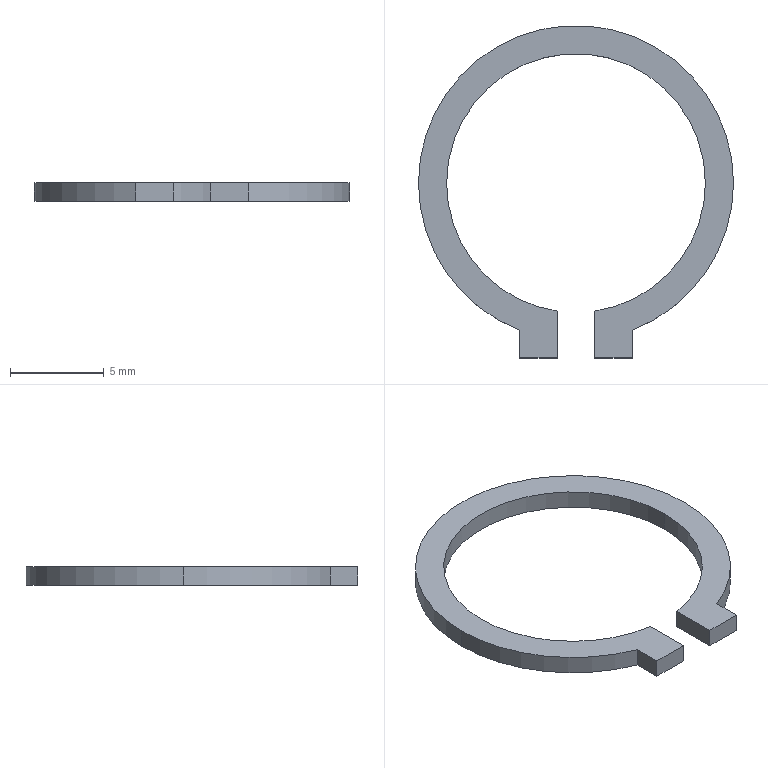Part | STEP file | Outer clip | 1 solid | 14 faces | box 16.8 x 17.727 x 1 mm | volume 73.853 mm3 | plane 8 | cylinder 6 | commonest cylinder face diameters 13.8 x3 16.8 x3
STEP:
#1=CARTESIAN_POINT('',(0.,0.,0.));
#2=DIRECTION('',(0.,0.,1.));
#3=DIRECTION('',(1.,0.,0.));
#4=AXIS2_PLACEMENT_3D('',#1,#2,#3);
#5=CARTESIAN_POINT('',(1.,-6.827,0.));
#6=VERTEX_POINT('',#5);
#7=CARTESIAN_POINT('',(1.,-6.827,1.));
#8=VERTEX_POINT('',#7);
#9=CARTESIAN_POINT('',(1.,-6.827,0.));
#10=DIRECTION('',(0.,0.,1.));
#11=VECTOR('',#10,1.);
#12=LINE('',#9,#11);
#13=CARTESIAN_POINT('',(0.,0.,1.));
#14=DIRECTION('',(0.,0.,-1.));
#15=DIRECTION('',(-1.,0.,0.));
#16=AXIS2_PLACEMENT_3D('',#13,#14,#15);
#17=CYLINDRICAL_SURFACE('',#16,6.9);
#18=CARTESIAN_POINT('',(4.567,1.));
#19=DIRECTION('',(0.,-1.));
#20=VECTOR('',#19,1.);
#21=LINE('',#18,#20);
#22=(GEOMETRIC_REPRESENTATION_CONTEXT(2)PARAMETRIC_REPRESENTATION_CONTEXT()REPRESENTATION_CONTEXT('',''));
#23=DEFINITIONAL_REPRESENTATION('',(#21),#22);
#24=PCURVE('',#17,#23);
#25=CARTESIAN_POINT('',(1.,-5.62,0.));
#26=DIRECTION('',(1.,0.,0.));
#27=DIRECTION('',(0.,1.,0.));
#28=AXIS2_PLACEMENT_3D('',#25,#26,#27);
#29=PLANE('',#28);
#30=CARTESIAN_POINT('',(-1.207,0.));
#31=DIRECTION('',(0.,1.));
#32=VECTOR('',#31,1.);
#33=LINE('',#30,#32);
#34=(GEOMETRIC_REPRESENTATION_CONTEXT(2)PARAMETRIC_REPRESENTATION_CONTEXT()REPRESENTATION_CONTEXT('',''));
#35=DEFINITIONAL_REPRESENTATION('',(#33),#34);
#36=PCURVE('',#29,#35);
#37=SURFACE_CURVE('',#12,(#24,#36),.PCURVE_S1.);
#38=EDGE_CURVE('',#6,#8,#37,.T.);
#39=ORIENTED_EDGE('',*,*,#38,.F.);
#40=CARTESIAN_POINT('',(6.9,0.,0.));
#41=VERTEX_POINT('',#40);
#42=CARTESIAN_POINT('',(0.,0.,0.));
#43=DIRECTION('',(0.,0.,-1.));
#44=DIRECTION('',(-1.,0.,0.));
#45=AXIS2_PLACEMENT_3D('',#42,#43,#44);
#46=CIRCLE('',#45,6.9);
#47=CARTESIAN_POINT('',(0.,1.));
#48=DIRECTION('',(1.,0.));
#49=VECTOR('',#48,1.);
#50=LINE('',#47,#49);
#51=(GEOMETRIC_REPRESENTATION_CONTEXT(2)PARAMETRIC_REPRESENTATION_CONTEXT()REPRESENTATION_CONTEXT('',''));
#52=DEFINITIONAL_REPRESENTATION('',(#50),#51);
#53=PCURVE('',#17,#52);
#54=CARTESIAN_POINT('',(0.,0.,0.));
#55=DIRECTION('',(0.,0.,1.));
#56=DIRECTION('',(1.,0.,0.));
#57=AXIS2_PLACEMENT_3D('',#54,#55,#56);
#58=PLANE('',#57);
#59=CARTESIAN_POINT('',(-6.9,0.));
#60=CARTESIAN_POINT('',(-6.9,11.951));
#61=CARTESIAN_POINT('',(3.45,5.976));
#62=CARTESIAN_POINT('',(13.8,0.));
#63=CARTESIAN_POINT('',(3.45,-5.976));
#64=CARTESIAN_POINT('',(-6.9,-11.951));
#65=CARTESIAN_POINT('',(-6.9,0.));
#66=(BOUNDED_CURVE()B_SPLINE_CURVE(2,(#59,#60,#61,#62,#63,#64,#65),.UNSPECIFIED.,.T.,.F.)B_SPLINE_CURVE_WITH_KNOTS((1,2,2,2,2,1),(-2.094,0.,2.094,4.189,6.283,8.378),.UNSPECIFIED.)CURVE()GEOMETRIC_REPRESENTATION_ITEM()RATIONAL_B_SPLINE_CURVE((1.,0.5,1.,0.5,1.,0.5,1.))REPRESENTATION_ITEM(''));
#67=(GEOMETRIC_REPRESENTATION_CONTEXT(2)PARAMETRIC_REPRESENTATION_CONTEXT()REPRESENTATION_CONTEXT('',''));
#68=DEFINITIONAL_REPRESENTATION('',(#66),#67);
#69=PCURVE('',#58,#68);
#70=SURFACE_CURVE('',#46,(#53,#69),.PCURVE_S1.);
#71=EDGE_CURVE('',#41,#6,#70,.T.);
#72=ORIENTED_EDGE('',*,*,#71,.F.);
#73=CARTESIAN_POINT('',(6.9,0.,1.));
#74=VERTEX_POINT('',#73);
#75=CARTESIAN_POINT('',(6.9,0.,1.));
#76=DIRECTION('',(0.,0.,-1.));
#77=VECTOR('',#76,1.);
#78=LINE('',#75,#77);
#79=CARTESIAN_POINT('',(3.142,0.));
#80=DIRECTION('',(0.,1.));
#81=VECTOR('',#80,1.);
#82=LINE('',#79,#81);
#83=(GEOMETRIC_REPRESENTATION_CONTEXT(2)PARAMETRIC_REPRESENTATION_CONTEXT()REPRESENTATION_CONTEXT('',''));
#84=DEFINITIONAL_REPRESENTATION('',(#82),#83);
#85=PCURVE('',#17,#84);
#86=CARTESIAN_POINT('',(0.,0.,1.));
#87=DIRECTION('',(0.,0.,-1.));
#88=DIRECTION('',(-1.,0.,0.));
#89=AXIS2_PLACEMENT_3D('',#86,#87,#88);
#90=CYLINDRICAL_SURFACE('',#89,6.9);
#91=CARTESIAN_POINT('',(3.142,0.));
#92=DIRECTION('',(0.,1.));
#93=VECTOR('',#92,1.);
#94=LINE('',#91,#93);
#95=(GEOMETRIC_REPRESENTATION_CONTEXT(2)PARAMETRIC_REPRESENTATION_CONTEXT()REPRESENTATION_CONTEXT('',''));
#96=DEFINITIONAL_REPRESENTATION('',(#94),#95);
#97=PCURVE('',#90,#96);
#98=SURFACE_CURVE('',#78,(#85,#97),.PCURVE_S1.);
#99=EDGE_CURVE('',#74,#41,#98,.T.);
#100=ORIENTED_EDGE('',*,*,#99,.F.);
#101=CARTESIAN_POINT('',(0.,0.,1.));
#102=DIRECTION('',(0.,0.,-1.));
#103=DIRECTION('',(-1.,0.,0.));
#104=AXIS2_PLACEMENT_3D('',#101,#102,#103);
#105=CIRCLE('',#104,6.9);
#106=CARTESIAN_POINT('',(0.,0.));
#107=DIRECTION('',(1.,0.));
#108=VECTOR('',#107,1.);
#109=LINE('',#106,#108);
#110=(GEOMETRIC_REPRESENTATION_CONTEXT(2)PARAMETRIC_REPRESENTATION_CONTEXT()REPRESENTATION_CONTEXT('',''));
#111=DEFINITIONAL_REPRESENTATION('',(#109),#110);
#112=PCURVE('',#17,#111);
#113=CARTESIAN_POINT('',(0.,0.,1.));
#114=DIRECTION('',(0.,0.,1.));
#115=DIRECTION('',(1.,0.,0.));
#116=AXIS2_PLACEMENT_3D('',#113,#114,#115);
#117=PLANE('',#116);
#118=CARTESIAN_POINT('',(-6.9,0.));
#119=CARTESIAN_POINT('',(-6.9,11.951));
#120=CARTESIAN_POINT('',(3.45,5.976));
#121=CARTESIAN_POINT('',(13.8,0.));
#122=CARTESIAN_POINT('',(3.45,-5.976));
#123=CARTESIAN_POINT('',(-6.9,-11.951));
#124=CARTESIAN_POINT('',(-6.9,0.));
#125=(BOUNDED_CURVE()B_SPLINE_CURVE(2,(#118,#119,#120,#121,#122,#123,#124),.UNSPECIFIED.,.T.,.F.)B_SPLINE_CURVE_WITH_KNOTS((1,2,2,2,2,1),(-2.094,0.,2.094,4.189,6.283,8.378),.UNSPECIFIED.)CURVE()GEOMETRIC_REPRESENTATION_ITEM()RATIONAL_B_SPLINE_CURVE((1.,0.5,1.,0.5,1.,0.5,1.))REPRESENTATION_ITEM(''));
#126=(GEOMETRIC_REPRESENTATION_CONTEXT(2)PARAMETRIC_REPRESENTATION_CONTEXT()REPRESENTATION_CONTEXT('',''));
#127=DEFINITIONAL_REPRESENTATION('',(#125),#126);
#128=PCURVE('',#117,#127);
#129=SURFACE_CURVE('',#105,(#112,#128),.PCURVE_S1.);
#130=EDGE_CURVE('',#74,#8,#129,.T.);
#131=ORIENTED_EDGE('',*,*,#130,.T.);
#132=EDGE_LOOP('',(#39,#72,#100,#131));
#133=FACE_BOUND('',#132,.F.);
#134=ADVANCED_FACE('',(#133),#17,.F.);
#135=CARTESIAN_POINT('',(-6.9,0.,0.));
#136=VERTEX_POINT('',#135);
#137=CARTESIAN_POINT('',(0.,0.,0.));
#138=DIRECTION('',(0.,0.,-1.));
#139=DIRECTION('',(-1.,0.,0.));
#140=AXIS2_PLACEMENT_3D('',#137,#138,#139);
#141=CIRCLE('',#140,6.9);
#142=CARTESIAN_POINT('',(0.,1.));
#143=DIRECTION('',(1.,0.));
#144=VECTOR('',#143,1.);
#145=LINE('',#142,#144);
#146=(GEOMETRIC_REPRESENTATION_CONTEXT(2)PARAMETRIC_REPRESENTATION_CONTEXT()REPRESENTATION_CONTEXT('',''));
#147=DEFINITIONAL_REPRESENTATION('',(#145),#146);
#148=PCURVE('',#90,#147);
#149=CARTESIAN_POINT('',(-6.9,0.));
#150=CARTESIAN_POINT('',(-6.9,11.951));
#151=CARTESIAN_POINT('',(3.45,5.976));
#152=CARTESIAN_POINT('',(13.8,0.));
#153=CARTESIAN_POINT('',(3.45,-5.976));
#154=CARTESIAN_POINT('',(-6.9,-11.951));
#155=CARTESIAN_POINT('',(-6.9,0.));
#156=(BOUNDED_CURVE()B_SPLINE_CURVE(2,(#149,#150,#151,#152,#153,#154,#155),.UNSPECIFIED.,.T.,.F.)B_SPLINE_CURVE_WITH_KNOTS((1,2,2,2,2,1),(-2.094,0.,2.094,4.189,6.283,8.378),.UNSPECIFIED.)CURVE()GEOMETRIC_REPRESENTATION_ITEM()RATIONAL_B_SPLINE_CURVE((1.,0.5,1.,0.5,1.,0.5,1.))REPRESENTATION_ITEM(''));
#157=(GEOMETRIC_REPRESENTATION_CONTEXT(2)PARAMETRIC_REPRESENTATION_CONTEXT()REPRESENTATION_CONTEXT('',''));
#158=DEFINITIONAL_REPRESENTATION('',(#156),#157);
#159=PCURVE('',#58,#158);
#160=SURFACE_CURVE('',#141,(#148,#159),.PCURVE_S1.);
#161=EDGE_CURVE('',#136,#41,#160,.T.);
#162=ORIENTED_EDGE('',*,*,#161,.F.);
#163=CARTESIAN_POINT('',(-6.9,0.,1.));
#164=VERTEX_POINT('',#163);
#165=CARTESIAN_POINT('',(-6.9,0.,1.));
#166=DIRECTION('',(0.,0.,-1.));
#167=VECTOR('',#166,1.);
#168=LINE('',#165,#167);
#169=CARTESIAN_POINT('',(0.,0.));
#170=DIRECTION('',(0.,1.));
#171=VECTOR('',#170,1.);
#172=LINE('',#169,#171);
#173=(GEOMETRIC_REPRESENTATION_CONTEXT(2)PARAMETRIC_REPRESENTATION_CONTEXT()REPRESENTATION_CONTEXT('',''));
#174=DEFINITIONAL_REPRESENTATION('',(#172),#173);
#175=PCURVE('',#90,#174);
#176=CARTESIAN_POINT('',(0.,0.,1.));
#177=DIRECTION('',(0.,0.,-1.));
#178=DIRECTION('',(-1.,0.,0.));
#179=AXIS2_PLACEMENT_3D('',#176,#177,#178);
#180=CYLINDRICAL_SURFACE('',#179,6.9);
#181=CARTESIAN_POINT('',(6.283,0.));
#182=DIRECTION('',(0.,1.));
#183=VECTOR('',#182,1.);
#184=LINE('',#181,#183);
#185=(GEOMETRIC_REPRESENTATION_CONTEXT(2)PARAMETRIC_REPRESENTATION_CONTEXT()REPRESENTATION_CONTEXT('',''));
#186=DEFINITIONAL_REPRESENTATION('',(#184),#185);
#187=PCURVE('',#180,#186);
#188=SURFACE_CURVE('',#168,(#175,#187),.PCURVE_S1.);
#189=EDGE_CURVE('',#164,#136,#188,.T.);
#190=ORIENTED_EDGE('',*,*,#189,.F.);
#191=CARTESIAN_POINT('',(0.,0.,1.));
#192=DIRECTION('',(0.,0.,-1.));
#193=DIRECTION('',(-1.,0.,0.));
#194=AXIS2_PLACEMENT_3D('',#191,#192,#193);
#195=CIRCLE('',#194,6.9);
#196=CARTESIAN_POINT('',(0.,0.));
#197=DIRECTION('',(1.,0.));
#198=VECTOR('',#197,1.);
#199=LINE('',#196,#198);
#200=(GEOMETRIC_REPRESENTATION_CONTEXT(2)PARAMETRIC_REPRESENTATION_CONTEXT()REPRESENTATION_CONTEXT('',''));
#201=DEFINITIONAL_REPRESENTATION('',(#199),#200);
#202=PCURVE('',#90,#201);
#203=CARTESIAN_POINT('',(-6.9,0.));
#204=CARTESIAN_POINT('',(-6.9,11.951));
#205=CARTESIAN_POINT('',(3.45,5.976));
#206=CARTESIAN_POINT('',(13.8,0.));
#207=CARTESIAN_POINT('',(3.45,-5.976));
#208=CARTESIAN_POINT('',(-6.9,-11.951));
#209=CARTESIAN_POINT('',(-6.9,0.));
#210=(BOUNDED_CURVE()B_SPLINE_CURVE(2,(#203,#204,#205,#206,#207,#208,#209),.UNSPECIFIED.,.T.,.F.)B_SPLINE_CURVE_WITH_KNOTS((1,2,2,2,2,1),(-2.094,0.,2.094,4.189,6.283,8.378),.UNSPECIFIED.)CURVE()GEOMETRIC_REPRESENTATION_ITEM()RATIONAL_B_SPLINE_CURVE((1.,0.5,1.,0.5,1.,0.5,1.))REPRESENTATION_ITEM(''));
#211=(GEOMETRIC_REPRESENTATION_CONTEXT(2)PARAMETRIC_REPRESENTATION_CONTEXT()REPRESENTATION_CONTEXT('',''));
#212=DEFINITIONAL_REPRESENTATION('',(#210),#211);
#213=PCURVE('',#117,#212);
#214=SURFACE_CURVE('',#195,(#202,#213),.PCURVE_S1.);
#215=EDGE_CURVE('',#164,#74,#214,.T.);
#216=ORIENTED_EDGE('',*,*,#215,.T.);
#217=ORIENTED_EDGE('',*,*,#99,.T.);
#218=EDGE_LOOP('',(#162,#190,#216,#217));
#219=FACE_BOUND('',#218,.F.);
#220=ADVANCED_FACE('',(#219),#90,.F.);
#221=CARTESIAN_POINT('',(-8.4,0.,1.));
#222=VERTEX_POINT('',#221);
#223=CARTESIAN_POINT('',(8.4,0.,1.));
#224=VERTEX_POINT('',#223);
#225=CARTESIAN_POINT('',(0.,0.,1.));
#226=DIRECTION('',(0.,0.,-1.));
#227=DIRECTION('',(-1.,0.,0.));
#228=AXIS2_PLACEMENT_3D('',#225,#226,#227);
#229=CIRCLE('',#228,8.4);
#230=CARTESIAN_POINT('',(0.,0.,1.));
#231=DIRECTION('',(0.,0.,-1.));
#232=DIRECTION('',(-1.,0.,0.));
#233=AXIS2_PLACEMENT_3D('',#230,#231,#232);
#234=CYLINDRICAL_SURFACE('',#233,8.4);
#235=CARTESIAN_POINT('',(0.,0.));
#236=DIRECTION('',(1.,0.));
#237=VECTOR('',#236,1.);
#238=LINE('',#235,#237);
#239=(GEOMETRIC_REPRESENTATION_CONTEXT(2)PARAMETRIC_REPRESENTATION_CONTEXT()REPRESENTATION_CONTEXT('',''));
#240=DEFINITIONAL_REPRESENTATION('',(#238),#239);
#241=PCURVE('',#234,#240);
#242=CARTESIAN_POINT('',(-8.4,0.));
#243=CARTESIAN_POINT('',(-8.4,14.549));
#244=CARTESIAN_POINT('',(4.2,7.275));
#245=CARTESIAN_POINT('',(16.8,0.));
#246=CARTESIAN_POINT('',(4.2,-7.275));
#247=CARTESIAN_POINT('',(-8.4,-14.549));
#248=CARTESIAN_POINT('',(-8.4,0.));
#249=(BOUNDED_CURVE()B_SPLINE_CURVE(2,(#242,#243,#244,#245,#246,#247,#248),.UNSPECIFIED.,.T.,.F.)B_SPLINE_CURVE_WITH_KNOTS((1,2,2,2,2,1),(-2.094,0.,2.094,4.189,6.283,8.378),.UNSPECIFIED.)CURVE()GEOMETRIC_REPRESENTATION_ITEM()RATIONAL_B_SPLINE_CURVE((1.,0.5,1.,0.5,1.,0.5,1.))REPRESENTATION_ITEM(''));
#250=(GEOMETRIC_REPRESENTATION_CONTEXT(2)PARAMETRIC_REPRESENTATION_CONTEXT()REPRESENTATION_CONTEXT('',''));
#251=DEFINITIONAL_REPRESENTATION('',(#249),#250);
#252=PCURVE('',#117,#251);
#253=SURFACE_CURVE('',#229,(#241,#252),.PCURVE_S1.);
#254=EDGE_CURVE('',#222,#224,#253,.T.);
#255=ORIENTED_EDGE('',*,*,#254,.T.);
#256=CARTESIAN_POINT('',(8.4,0.,0.));
#257=VERTEX_POINT('',#256);
#258=CARTESIAN_POINT('',(8.4,0.,1.));
#259=DIRECTION('',(0.,0.,-1.));
#260=VECTOR('',#259,1.);
#261=LINE('',#258,#260);
#262=CARTESIAN_POINT('',(3.142,0.));
#263=DIRECTION('',(0.,1.));
#264=VECTOR('',#263,1.);
#265=LINE('',#262,#264);
#266=(GEOMETRIC_REPRESENTATION_CONTEXT(2)PARAMETRIC_REPRESENTATION_CONTEXT()REPRESENTATION_CONTEXT('',''));
#267=DEFINITIONAL_REPRESENTATION('',(#265),#266);
#268=PCURVE('',#234,#267);
#269=CARTESIAN_POINT('',(0.,0.,1.));
#270=DIRECTION('',(0.,0.,-1.));
#271=DIRECTION('',(-1.,0.,0.));
#272=AXIS2_PLACEMENT_3D('',#269,#270,#271);
#273=CYLINDRICAL_SURFACE('',#272,8.4);
#274=CARTESIAN_POINT('',(3.142,0.));
#275=DIRECTION('',(0.,1.));
#276=VECTOR('',#275,1.);
#277=LINE('',#274,#276);
#278=(GEOMETRIC_REPRESENTATION_CONTEXT(2)PARAMETRIC_REPRESENTATION_CONTEXT()REPRESENTATION_CONTEXT('',''));
#279=DEFINITIONAL_REPRESENTATION('',(#277),#278);
#280=PCURVE('',#273,#279);
#281=SURFACE_CURVE('',#261,(#268,#280),.PCURVE_S1.);
#282=EDGE_CURVE('',#224,#257,#281,.T.);
#283=ORIENTED_EDGE('',*,*,#282,.T.);
#284=CARTESIAN_POINT('',(-8.4,0.,0.));
#285=VERTEX_POINT('',#284);
#286=CARTESIAN_POINT('',(0.,0.,0.));
#287=DIRECTION('',(0.,0.,1.));
#288=DIRECTION('',(-1.,0.,0.));
#289=AXIS2_PLACEMENT_3D('',#286,#287,#288);
#290=CIRCLE('',#289,8.4);
#291=CARTESIAN_POINT('',(6.283,1.));
#292=DIRECTION('',(-1.,0.));
#293=VECTOR('',#292,1.);
#294=LINE('',#291,#293);
#295=(GEOMETRIC_REPRESENTATION_CONTEXT(2)PARAMETRIC_REPRESENTATION_CONTEXT()REPRESENTATION_CONTEXT('',''));
#296=DEFINITIONAL_REPRESENTATION('',(#294),#295);
#297=PCURVE('',#234,#296);
#298=CARTESIAN_POINT('',(0.,0.));
#299=DIRECTION('',(-1.,0.));
#300=AXIS2_PLACEMENT_2D('',#298,#299);
#301=CIRCLE('',#300,8.4);
#302=(GEOMETRIC_REPRESENTATION_CONTEXT(2)PARAMETRIC_REPRESENTATION_CONTEXT()REPRESENTATION_CONTEXT('',''));
#303=DEFINITIONAL_REPRESENTATION('',(#301),#302);
#304=PCURVE('',#58,#303);
#305=SURFACE_CURVE('',#290,(#297,#304),.PCURVE_S1.);
#306=EDGE_CURVE('',#257,#285,#305,.T.);
#307=ORIENTED_EDGE('',*,*,#306,.T.);
#308=CARTESIAN_POINT('',(-8.4,0.,1.));
#309=DIRECTION('',(0.,0.,-1.));
#310=VECTOR('',#309,1.);
#311=LINE('',#308,#310);
#312=CARTESIAN_POINT('',(0.,0.));
#313=DIRECTION('',(0.,1.));
#314=VECTOR('',#313,1.);
#315=LINE('',#312,#314);
#316=(GEOMETRIC_REPRESENTATION_CONTEXT(2)PARAMETRIC_REPRESENTATION_CONTEXT()REPRESENTATION_CONTEXT('',''));
#317=DEFINITIONAL_REPRESENTATION('',(#315),#316);
#318=PCURVE('',#234,#317);
#319=CARTESIAN_POINT('',(0.,0.,1.));
#320=DIRECTION('',(0.,0.,-1.));
#321=DIRECTION('',(-1.,0.,0.));
#322=AXIS2_PLACEMENT_3D('',#319,#320,#321);
#323=CYLINDRICAL_SURFACE('',#322,8.4);
#324=CARTESIAN_POINT('',(6.283,0.));
#325=DIRECTION('',(0.,1.));
#326=VECTOR('',#325,1.);
#327=LINE('',#324,#326);
#328=(GEOMETRIC_REPRESENTATION_CONTEXT(2)PARAMETRIC_REPRESENTATION_CONTEXT()REPRESENTATION_CONTEXT('',''));
#329=DEFINITIONAL_REPRESENTATION('',(#327),#328);
#330=PCURVE('',#323,#329);
#331=SURFACE_CURVE('',#311,(#318,#330),.PCURVE_S1.);
#332=EDGE_CURVE('',#222,#285,#331,.T.);
#333=ORIENTED_EDGE('',*,*,#332,.F.);
#334=EDGE_LOOP('',(#255,#283,#307,#333));
#335=FACE_BOUND('',#334,.T.);
#336=ADVANCED_FACE('',(#335),#234,.T.);
#337=CARTESIAN_POINT('',(-3.,-7.846,1.));
#338=VERTEX_POINT('',#337);
#339=CARTESIAN_POINT('',(0.,0.,1.));
#340=DIRECTION('',(0.,0.,-1.));
#341=DIRECTION('',(-1.,0.,0.));
#342=AXIS2_PLACEMENT_3D('',#339,#340,#341);
#343=CIRCLE('',#342,8.4);
#344=CARTESIAN_POINT('',(0.,0.));
#345=DIRECTION('',(1.,0.));
#346=VECTOR('',#345,1.);
#347=LINE('',#344,#346);
#348=(GEOMETRIC_REPRESENTATION_CONTEXT(2)PARAMETRIC_REPRESENTATION_CONTEXT()REPRESENTATION_CONTEXT('',''));
#349=DEFINITIONAL_REPRESENTATION('',(#347),#348);
#350=PCURVE('',#323,#349);
#351=CARTESIAN_POINT('',(-8.4,0.));
#352=CARTESIAN_POINT('',(-8.4,14.549));
#353=CARTESIAN_POINT('',(4.2,7.275));
#354=CARTESIAN_POINT('',(16.8,0.));
#355=CARTESIAN_POINT('',(4.2,-7.275));
#356=CARTESIAN_POINT('',(-8.4,-14.549));
#357=CARTESIAN_POINT('',(-8.4,0.));
#358=(BOUNDED_CURVE()B_SPLINE_CURVE(2,(#351,#352,#353,#354,#355,#356,#357),.UNSPECIFIED.,.T.,.F.)B_SPLINE_CURVE_WITH_KNOTS((1,2,2,2,2,1),(-2.094,0.,2.094,4.189,6.283,8.378),.UNSPECIFIED.)CURVE()GEOMETRIC_REPRESENTATION_ITEM()RATIONAL_B_SPLINE_CURVE((1.,0.5,1.,0.5,1.,0.5,1.))REPRESENTATION_ITEM(''));
#359=(GEOMETRIC_REPRESENTATION_CONTEXT(2)PARAMETRIC_REPRESENTATION_CONTEXT()REPRESENTATION_CONTEXT('',''));
#360=DEFINITIONAL_REPRESENTATION('',(#358),#359);
#361=PCURVE('',#117,#360);
#362=SURFACE_CURVE('',#343,(#350,#361),.PCURVE_S1.);
#363=EDGE_CURVE('',#338,#222,#362,.T.);
#364=ORIENTED_EDGE('',*,*,#363,.T.);
#365=ORIENTED_EDGE('',*,*,#332,.T.);
#366=CARTESIAN_POINT('',(-3.,-7.846,0.));
#367=VERTEX_POINT('',#366);
#368=CARTESIAN_POINT('',(0.,0.,0.));
#369=DIRECTION('',(0.,0.,1.));
#370=DIRECTION('',(-1.,0.,0.));
#371=AXIS2_PLACEMENT_3D('',#368,#369,#370);
#372=CIRCLE('',#371,8.4);
#373=CARTESIAN_POINT('',(6.283,1.));
#374=DIRECTION('',(-1.,0.));
#375=VECTOR('',#374,1.);
#376=LINE('',#373,#375);
#377=(GEOMETRIC_REPRESENTATION_CONTEXT(2)PARAMETRIC_REPRESENTATION_CONTEXT()REPRESENTATION_CONTEXT('',''));
#378=DEFINITIONAL_REPRESENTATION('',(#376),#377);
#379=PCURVE('',#323,#378);
#380=CARTESIAN_POINT('',(0.,0.));
#381=DIRECTION('',(-1.,0.));
#382=AXIS2_PLACEMENT_2D('',#380,#381);
#383=CIRCLE('',#382,8.4);
#384=(GEOMETRIC_REPRESENTATION_CONTEXT(2)PARAMETRIC_REPRESENTATION_CONTEXT()REPRESENTATION_CONTEXT('',''));
#385=DEFINITIONAL_REPRESENTATION('',(#383),#384);
#386=PCURVE('',#58,#385);
#387=SURFACE_CURVE('',#372,(#379,#386),.PCURVE_S1.);
#388=EDGE_CURVE('',#285,#367,#387,.T.);
#389=ORIENTED_EDGE('',*,*,#388,.T.);
#390=CARTESIAN_POINT('',(-3.,-7.846,0.));
#391=DIRECTION('',(0.,0.,-1.));
#392=VECTOR('',#391,1.);
#393=LINE('',#390,#392);
#394=CARTESIAN_POINT('',(5.078,1.));
#395=DIRECTION('',(0.,1.));
#396=VECTOR('',#395,1.);
#397=LINE('',#394,#396);
#398=(GEOMETRIC_REPRESENTATION_CONTEXT(2)PARAMETRIC_REPRESENTATION_CONTEXT()REPRESENTATION_CONTEXT('',''));
#399=DEFINITIONAL_REPRESENTATION('',(#397),#398);
#400=PCURVE('',#323,#399);
#401=CARTESIAN_POINT('',(-3.,-6.827,0.));
#402=DIRECTION('',(-1.,0.,0.));
#403=DIRECTION('',(0.,-1.,0.));
#404=AXIS2_PLACEMENT_3D('',#401,#402,#403);
#405=PLANE('',#404);
#406=CARTESIAN_POINT('',(1.019,0.));
#407=DIRECTION('',(0.,-1.));
#408=VECTOR('',#407,1.);
#409=LINE('',#406,#408);
#410=(GEOMETRIC_REPRESENTATION_CONTEXT(2)PARAMETRIC_REPRESENTATION_CONTEXT()REPRESENTATION_CONTEXT('',''));
#411=DEFINITIONAL_REPRESENTATION('',(#409),#410);
#412=PCURVE('',#405,#411);
#413=SURFACE_CURVE('',#393,(#400,#412),.PCURVE_S1.);
#414=EDGE_CURVE('',#338,#367,#413,.T.);
#415=ORIENTED_EDGE('',*,*,#414,.F.);
#416=EDGE_LOOP('',(#364,#365,#389,#415));
#417=FACE_BOUND('',#416,.T.);
#418=ADVANCED_FACE('',(#417),#323,.T.);
#419=CARTESIAN_POINT('',(1.,-9.327,0.));
#420=VERTEX_POINT('',#419);
#421=CARTESIAN_POINT('',(1.,0.,0.));
#422=DIRECTION('',(0.,-1.,0.));
#423=VECTOR('',#422,1.);
#424=LINE('',#421,#423);
#425=CARTESIAN_POINT('',(1.,0.));
#426=DIRECTION('',(0.,-1.));
#427=VECTOR('',#426,1.);
#428=LINE('',#425,#427);
#429=(GEOMETRIC_REPRESENTATION_CONTEXT(2)PARAMETRIC_REPRESENTATION_CONTEXT()REPRESENTATION_CONTEXT('',''));
#430=DEFINITIONAL_REPRESENTATION('',(#428),#429);
#431=PCURVE('',#58,#430);
#432=CARTESIAN_POINT('',(5.62,0.));
#433=DIRECTION('',(-1.,0.));
#434=VECTOR('',#433,1.);
#435=LINE('',#432,#434);
#436=(GEOMETRIC_REPRESENTATION_CONTEXT(2)PARAMETRIC_REPRESENTATION_CONTEXT()REPRESENTATION_CONTEXT('',''));
#437=DEFINITIONAL_REPRESENTATION('',(#435),#436);
#438=PCURVE('',#29,#437);
#439=SURFACE_CURVE('',#424,(#431,#438),.PCURVE_S1.);
#440=EDGE_CURVE('',#6,#420,#439,.T.);
#441=ORIENTED_EDGE('',*,*,#440,.F.);
#442=ORIENTED_EDGE('',*,*,#71,.F.);
#443=ORIENTED_EDGE('',*,*,#161,.F.);
#444=CARTESIAN_POINT('',(-1.,-6.827,0.));
#445=VERTEX_POINT('',#444);
#446=CARTESIAN_POINT('',(0.,0.,0.));
#447=DIRECTION('',(0.,0.,-1.));
#448=DIRECTION('',(-1.,0.,0.));
#449=AXIS2_PLACEMENT_3D('',#446,#447,#448);
#450=CIRCLE('',#449,6.9);
#451=CARTESIAN_POINT('',(-6.9,0.));
#452=CARTESIAN_POINT('',(-6.9,11.951));
#453=CARTESIAN_POINT('',(3.45,5.976));
#454=CARTESIAN_POINT('',(13.8,0.));
#455=CARTESIAN_POINT('',(3.45,-5.976));
#456=CARTESIAN_POINT('',(-6.9,-11.951));
#457=CARTESIAN_POINT('',(-6.9,0.));
#458=(BOUNDED_CURVE()B_SPLINE_CURVE(2,(#451,#452,#453,#454,#455,#456,#457),.UNSPECIFIED.,.T.,.F.)B_SPLINE_CURVE_WITH_KNOTS((1,2,2,2,2,1),(-2.094,0.,2.094,4.189,6.283,8.378),.UNSPECIFIED.)CURVE()GEOMETRIC_REPRESENTATION_ITEM()RATIONAL_B_SPLINE_CURVE((1.,0.5,1.,0.5,1.,0.5,1.))REPRESENTATION_ITEM(''));
#459=(GEOMETRIC_REPRESENTATION_CONTEXT(2)PARAMETRIC_REPRESENTATION_CONTEXT()REPRESENTATION_CONTEXT('',''));
#460=DEFINITIONAL_REPRESENTATION('',(#458),#459);
#461=PCURVE('',#58,#460);
#462=CARTESIAN_POINT('',(0.,1.));
#463=DIRECTION('',(1.,0.));
#464=VECTOR('',#463,1.);
#465=LINE('',#462,#464);
#466=(GEOMETRIC_REPRESENTATION_CONTEXT(2)PARAMETRIC_REPRESENTATION_CONTEXT()REPRESENTATION_CONTEXT('',''));
#467=DEFINITIONAL_REPRESENTATION('',(#465),#466);
#468=PCURVE('',#180,#467);
#469=SURFACE_CURVE('',#450,(#461,#468),.PCURVE_S1.);
#470=EDGE_CURVE('',#445,#136,#469,.T.);
#471=ORIENTED_EDGE('',*,*,#470,.F.);
#472=CARTESIAN_POINT('',(-1.,-9.327,0.));
#473=VERTEX_POINT('',#472);
#474=CARTESIAN_POINT('',(-1.,0.,0.));
#475=DIRECTION('',(0.,1.,0.));
#476=VECTOR('',#475,1.);
#477=LINE('',#474,#476);
#478=CARTESIAN_POINT('',(-1.,0.));
#479=DIRECTION('',(0.,1.));
#480=VECTOR('',#479,1.);
#481=LINE('',#478,#480);
#482=(GEOMETRIC_REPRESENTATION_CONTEXT(2)PARAMETRIC_REPRESENTATION_CONTEXT()REPRESENTATION_CONTEXT('',''));
#483=DEFINITIONAL_REPRESENTATION('',(#481),#482);
#484=PCURVE('',#58,#483);
#485=CARTESIAN_POINT('',(-1.,-5.62,0.));
#486=DIRECTION('',(-1.,0.,0.));
#487=DIRECTION('',(0.,-1.,0.));
#488=AXIS2_PLACEMENT_3D('',#485,#486,#487);
#489=PLANE('',#488);
#490=CARTESIAN_POINT('',(-5.62,0.));
#491=DIRECTION('',(-1.,0.));
#492=VECTOR('',#491,1.);
#493=LINE('',#490,#492);
#494=(GEOMETRIC_REPRESENTATION_CONTEXT(2)PARAMETRIC_REPRESENTATION_CONTEXT()REPRESENTATION_CONTEXT('',''));
#495=DEFINITIONAL_REPRESENTATION('',(#493),#494);
#496=PCURVE('',#489,#495);
#497=SURFACE_CURVE('',#477,(#484,#496),.PCURVE_S1.);
#498=EDGE_CURVE('',#473,#445,#497,.T.);
#499=ORIENTED_EDGE('',*,*,#498,.F.);
#500=CARTESIAN_POINT('',(-3.,-9.327,0.));
#501=VERTEX_POINT('',#500);
#502=CARTESIAN_POINT('',(0.,-9.327,0.));
#503=DIRECTION('',(1.,0.,0.));
#504=VECTOR('',#503,1.);
#505=LINE('',#502,#504);
#506=CARTESIAN_POINT('',(0.,-9.327));
#507=DIRECTION('',(1.,0.));
#508=VECTOR('',#507,1.);
#509=LINE('',#506,#508);
#510=(GEOMETRIC_REPRESENTATION_CONTEXT(2)PARAMETRIC_REPRESENTATION_CONTEXT()REPRESENTATION_CONTEXT('',''));
#511=DEFINITIONAL_REPRESENTATION('',(#509),#510);
#512=PCURVE('',#58,#511);
#513=CARTESIAN_POINT('',(-1.,-9.327,0.));
#514=DIRECTION('',(0.,-1.,0.));
#515=DIRECTION('',(0.,0.,-1.));
#516=AXIS2_PLACEMENT_3D('',#513,#514,#515);
#517=PLANE('',#516);
#518=CARTESIAN_POINT('',(0.,1.));
#519=DIRECTION('',(0.,1.));
#520=VECTOR('',#519,1.);
#521=LINE('',#518,#520);
#522=(GEOMETRIC_REPRESENTATION_CONTEXT(2)PARAMETRIC_REPRESENTATION_CONTEXT()REPRESENTATION_CONTEXT('',''));
#523=DEFINITIONAL_REPRESENTATION('',(#521),#522);
#524=PCURVE('',#517,#523);
#525=SURFACE_CURVE('',#505,(#512,#524),.PCURVE_S1.);
#526=EDGE_CURVE('',#501,#473,#525,.T.);
#527=ORIENTED_EDGE('',*,*,#526,.F.);
#528=CARTESIAN_POINT('',(-3.,0.,0.));
#529=DIRECTION('',(0.,-1.,0.));
#530=VECTOR('',#529,1.);
#531=LINE('',#528,#530);
#532=CARTESIAN_POINT('',(-3.,0.));
#533=DIRECTION('',(0.,-1.));
#534=VECTOR('',#533,1.);
#535=LINE('',#532,#534);
#536=(GEOMETRIC_REPRESENTATION_CONTEXT(2)PARAMETRIC_REPRESENTATION_CONTEXT()REPRESENTATION_CONTEXT('',''));
#537=DEFINITIONAL_REPRESENTATION('',(#535),#536);
#538=PCURVE('',#58,#537);
#539=CARTESIAN_POINT('',(-6.827,0.));
#540=DIRECTION('',(1.,0.));
#541=VECTOR('',#540,1.);
#542=LINE('',#539,#541);
#543=(GEOMETRIC_REPRESENTATION_CONTEXT(2)PARAMETRIC_REPRESENTATION_CONTEXT()REPRESENTATION_CONTEXT('',''));
#544=DEFINITIONAL_REPRESENTATION('',(#542),#543);
#545=PCURVE('',#405,#544);
#546=SURFACE_CURVE('',#531,(#538,#545),.PCURVE_S1.);
#547=EDGE_CURVE('',#367,#501,#546,.T.);
#548=ORIENTED_EDGE('',*,*,#547,.F.);
#549=ORIENTED_EDGE('',*,*,#388,.F.);
#550=ORIENTED_EDGE('',*,*,#306,.F.);
#551=CARTESIAN_POINT('',(3.,-7.846,0.));
#552=VERTEX_POINT('',#551);
#553=CARTESIAN_POINT('',(0.,0.,0.));
#554=DIRECTION('',(0.,0.,1.));
#555=DIRECTION('',(-1.,0.,0.));
#556=AXIS2_PLACEMENT_3D('',#553,#554,#555);
#557=CIRCLE('',#556,8.4);
#558=CARTESIAN_POINT('',(0.,0.));
#559=DIRECTION('',(-1.,0.));
#560=AXIS2_PLACEMENT_2D('',#558,#559);
#561=CIRCLE('',#560,8.4);
#562=(GEOMETRIC_REPRESENTATION_CONTEXT(2)PARAMETRIC_REPRESENTATION_CONTEXT()REPRESENTATION_CONTEXT('',''));
#563=DEFINITIONAL_REPRESENTATION('',(#561),#562);
#564=PCURVE('',#58,#563);
#565=CARTESIAN_POINT('',(6.283,1.));
#566=DIRECTION('',(-1.,0.));
#567=VECTOR('',#566,1.);
#568=LINE('',#565,#567);
#569=(GEOMETRIC_REPRESENTATION_CONTEXT(2)PARAMETRIC_REPRESENTATION_CONTEXT()REPRESENTATION_CONTEXT('',''));
#570=DEFINITIONAL_REPRESENTATION('',(#568),#569);
#571=PCURVE('',#273,#570);
#572=SURFACE_CURVE('',#557,(#564,#571),.PCURVE_S1.);
#573=EDGE_CURVE('',#552,#257,#572,.T.);
#574=ORIENTED_EDGE('',*,*,#573,.F.);
#575=CARTESIAN_POINT('',(3.,-9.327,0.));
#576=VERTEX_POINT('',#575);
#577=CARTESIAN_POINT('',(3.,0.,0.));
#578=DIRECTION('',(0.,1.,0.));
#579=VECTOR('',#578,1.);
#580=LINE('',#577,#579);
#581=CARTESIAN_POINT('',(3.,0.));
#582=DIRECTION('',(0.,1.));
#583=VECTOR('',#582,1.);
#584=LINE('',#581,#583);
#585=(GEOMETRIC_REPRESENTATION_CONTEXT(2)PARAMETRIC_REPRESENTATION_CONTEXT()REPRESENTATION_CONTEXT('',''));
#586=DEFINITIONAL_REPRESENTATION('',(#584),#585);
#587=PCURVE('',#58,#586);
#588=CARTESIAN_POINT('',(3.,-6.827,0.));
#589=DIRECTION('',(1.,0.,0.));
#590=DIRECTION('',(0.,1.,0.));
#591=AXIS2_PLACEMENT_3D('',#588,#589,#590);
#592=PLANE('',#591);
#593=CARTESIAN_POINT('',(6.827,0.));
#594=DIRECTION('',(1.,0.));
#595=VECTOR('',#594,1.);
#596=LINE('',#593,#595);
#597=(GEOMETRIC_REPRESENTATION_CONTEXT(2)PARAMETRIC_REPRESENTATION_CONTEXT()REPRESENTATION_CONTEXT('',''));
#598=DEFINITIONAL_REPRESENTATION('',(#596),#597);
#599=PCURVE('',#592,#598);
#600=SURFACE_CURVE('',#580,(#587,#599),.PCURVE_S1.);
#601=EDGE_CURVE('',#576,#552,#600,.T.);
#602=ORIENTED_EDGE('',*,*,#601,.F.);
#603=CARTESIAN_POINT('',(0.,-9.327,0.));
#604=DIRECTION('',(1.,0.,0.));
#605=VECTOR('',#604,1.);
#606=LINE('',#603,#605);
#607=CARTESIAN_POINT('',(0.,-9.327));
#608=DIRECTION('',(1.,0.));
#609=VECTOR('',#608,1.);
#610=LINE('',#607,#609);
#611=(GEOMETRIC_REPRESENTATION_CONTEXT(2)PARAMETRIC_REPRESENTATION_CONTEXT()REPRESENTATION_CONTEXT('',''));
#612=DEFINITIONAL_REPRESENTATION('',(#610),#611);
#613=PCURVE('',#58,#612);
#614=CARTESIAN_POINT('',(1.,-9.327,0.));
#615=DIRECTION('',(0.,-1.,0.));
#616=DIRECTION('',(0.,0.,-1.));
#617=AXIS2_PLACEMENT_3D('',#614,#615,#616);
#618=PLANE('',#617);
#619=CARTESIAN_POINT('',(0.,-1.));
#620=DIRECTION('',(0.,1.));
#621=VECTOR('',#620,1.);
#622=LINE('',#619,#621);
#623=(GEOMETRIC_REPRESENTATION_CONTEXT(2)PARAMETRIC_REPRESENTATION_CONTEXT()REPRESENTATION_CONTEXT('',''));
#624=DEFINITIONAL_REPRESENTATION('',(#622),#623);
#625=PCURVE('',#618,#624);
#626=SURFACE_CURVE('',#606,(#613,#625),.PCURVE_S1.);
#627=EDGE_CURVE('',#420,#576,#626,.T.);
#628=ORIENTED_EDGE('',*,*,#627,.F.);
#629=EDGE_LOOP('',(#441,#442,#443,#471,#499,#527,#548,#549,#550,#574,#602,#628));
#630=FACE_BOUND('',#629,.T.);
#631=ADVANCED_FACE('',(#630),#58,.F.);
#632=ORIENTED_EDGE('',*,*,#38,.F.);
#633=ORIENTED_EDGE('',*,*,#440,.T.);
#634=CARTESIAN_POINT('',(1.,-9.327,1.));
#635=VERTEX_POINT('',#634);
#636=CARTESIAN_POINT('',(1.,-9.327,0.));
#637=DIRECTION('',(0.,0.,-1.));
#638=VECTOR('',#637,1.);
#639=LINE('',#636,#638);
#640=CARTESIAN_POINT('',(-3.707,0.));
#641=DIRECTION('',(0.,-1.));
#642=VECTOR('',#641,1.);
#643=LINE('',#640,#642);
#644=(GEOMETRIC_REPRESENTATION_CONTEXT(2)PARAMETRIC_REPRESENTATION_CONTEXT()REPRESENTATION_CONTEXT('',''));
#645=DEFINITIONAL_REPRESENTATION('',(#643),#644);
#646=PCURVE('',#29,#645);
#647=CARTESIAN_POINT('',(0.,0.));
#648=DIRECTION('',(1.,0.));
#649=VECTOR('',#648,1.);
#650=LINE('',#647,#649);
#651=(GEOMETRIC_REPRESENTATION_CONTEXT(2)PARAMETRIC_REPRESENTATION_CONTEXT()REPRESENTATION_CONTEXT('',''));
#652=DEFINITIONAL_REPRESENTATION('',(#650),#651);
#653=PCURVE('',#618,#652);
#654=SURFACE_CURVE('',#639,(#646,#653),.PCURVE_S1.);
#655=EDGE_CURVE('',#635,#420,#654,.T.);
#656=ORIENTED_EDGE('',*,*,#655,.F.);
#657=CARTESIAN_POINT('',(1.,-5.62,1.));
#658=DIRECTION('',(0.,-1.,0.));
#659=VECTOR('',#658,1.);
#660=LINE('',#657,#659);
#661=CARTESIAN_POINT('',(0.,1.));
#662=DIRECTION('',(-1.,0.));
#663=VECTOR('',#662,1.);
#664=LINE('',#661,#663);
#665=(GEOMETRIC_REPRESENTATION_CONTEXT(2)PARAMETRIC_REPRESENTATION_CONTEXT()REPRESENTATION_CONTEXT('',''));
#666=DEFINITIONAL_REPRESENTATION('',(#664),#665);
#667=PCURVE('',#29,#666);
#668=CARTESIAN_POINT('',(1.,-5.62));
#669=DIRECTION('',(0.,-1.));
#670=VECTOR('',#669,1.);
#671=LINE('',#668,#670);
#672=(GEOMETRIC_REPRESENTATION_CONTEXT(2)PARAMETRIC_REPRESENTATION_CONTEXT()REPRESENTATION_CONTEXT('',''));
#673=DEFINITIONAL_REPRESENTATION('',(#671),#672);
#674=PCURVE('',#117,#673);
#675=SURFACE_CURVE('',#660,(#667,#674),.PCURVE_S1.);
#676=EDGE_CURVE('',#8,#635,#675,.T.);
#677=ORIENTED_EDGE('',*,*,#676,.F.);
#678=EDGE_LOOP('',(#632,#633,#656,#677));
#679=FACE_BOUND('',#678,.T.);
#680=ADVANCED_FACE('',(#679),#29,.F.);
#681=ORIENTED_EDGE('',*,*,#470,.F.);
#682=CARTESIAN_POINT('',(-1.,-6.827,1.));
#683=VERTEX_POINT('',#682);
#684=CARTESIAN_POINT('',(-1.,-6.827,1.));
#685=DIRECTION('',(0.,0.,1.));
#686=VECTOR('',#685,1.);
#687=LINE('',#684,#686);
#688=CARTESIAN_POINT('',(4.858,0.));
#689=DIRECTION('',(0.,-1.));
#690=VECTOR('',#689,1.);
#691=LINE('',#688,#690);
#692=(GEOMETRIC_REPRESENTATION_CONTEXT(2)PARAMETRIC_REPRESENTATION_CONTEXT()REPRESENTATION_CONTEXT('',''));
#693=DEFINITIONAL_REPRESENTATION('',(#691),#692);
#694=PCURVE('',#180,#693);
#695=CARTESIAN_POINT('',(1.207,1.));
#696=DIRECTION('',(0.,1.));
#697=VECTOR('',#696,1.);
#698=LINE('',#695,#697);
#699=(GEOMETRIC_REPRESENTATION_CONTEXT(2)PARAMETRIC_REPRESENTATION_CONTEXT()REPRESENTATION_CONTEXT('',''));
#700=DEFINITIONAL_REPRESENTATION('',(#698),#699);
#701=PCURVE('',#489,#700);
#702=SURFACE_CURVE('',#687,(#694,#701),.PCURVE_S1.);
#703=EDGE_CURVE('',#445,#683,#702,.T.);
#704=ORIENTED_EDGE('',*,*,#703,.T.);
#705=CARTESIAN_POINT('',(0.,0.,1.));
#706=DIRECTION('',(0.,0.,-1.));
#707=DIRECTION('',(-1.,0.,0.));
#708=AXIS2_PLACEMENT_3D('',#705,#706,#707);
#709=CIRCLE('',#708,6.9);
#710=CARTESIAN_POINT('',(0.,0.));
#711=DIRECTION('',(1.,0.));
#712=VECTOR('',#711,1.);
#713=LINE('',#710,#712);
#714=(GEOMETRIC_REPRESENTATION_CONTEXT(2)PARAMETRIC_REPRESENTATION_CONTEXT()REPRESENTATION_CONTEXT('',''));
#715=DEFINITIONAL_REPRESENTATION('',(#713),#714);
#716=PCURVE('',#180,#715);
#717=CARTESIAN_POINT('',(-6.9,0.));
#718=CARTESIAN_POINT('',(-6.9,11.951));
#719=CARTESIAN_POINT('',(3.45,5.976));
#720=CARTESIAN_POINT('',(13.8,0.));
#721=CARTESIAN_POINT('',(3.45,-5.976));
#722=CARTESIAN_POINT('',(-6.9,-11.951));
#723=CARTESIAN_POINT('',(-6.9,0.));
#724=(BOUNDED_CURVE()B_SPLINE_CURVE(2,(#717,#718,#719,#720,#721,#722,#723),.UNSPECIFIED.,.T.,.F.)B_SPLINE_CURVE_WITH_KNOTS((1,2,2,2,2,1),(-2.094,0.,2.094,4.189,6.283,8.378),.UNSPECIFIED.)CURVE()GEOMETRIC_REPRESENTATION_ITEM()RATIONAL_B_SPLINE_CURVE((1.,0.5,1.,0.5,1.,0.5,1.))REPRESENTATION_ITEM(''));
#725=(GEOMETRIC_REPRESENTATION_CONTEXT(2)PARAMETRIC_REPRESENTATION_CONTEXT()REPRESENTATION_CONTEXT('',''));
#726=DEFINITIONAL_REPRESENTATION('',(#724),#725);
#727=PCURVE('',#117,#726);
#728=SURFACE_CURVE('',#709,(#716,#727),.PCURVE_S1.);
#729=EDGE_CURVE('',#683,#164,#728,.T.);
#730=ORIENTED_EDGE('',*,*,#729,.T.);
#731=ORIENTED_EDGE('',*,*,#189,.T.);
#732=EDGE_LOOP('',(#681,#704,#730,#731));
#733=FACE_BOUND('',#732,.F.);
#734=ADVANCED_FACE('',(#733),#180,.F.);
#735=ORIENTED_EDGE('',*,*,#703,.T.);
#736=CARTESIAN_POINT('',(-1.,-9.327,1.));
#737=VERTEX_POINT('',#736);
#738=CARTESIAN_POINT('',(-1.,-5.62,1.));
#739=DIRECTION('',(0.,1.,0.));
#740=VECTOR('',#739,1.);
#741=LINE('',#738,#740);
#742=CARTESIAN_POINT('',(0.,1.));
#743=DIRECTION('',(-1.,0.));
#744=VECTOR('',#743,1.);
#745=LINE('',#742,#744);
#746=(GEOMETRIC_REPRESENTATION_CONTEXT(2)PARAMETRIC_REPRESENTATION_CONTEXT()REPRESENTATION_CONTEXT('',''));
#747=DEFINITIONAL_REPRESENTATION('',(#745),#746);
#748=PCURVE('',#489,#747);
#749=CARTESIAN_POINT('',(-1.,-5.62));
#750=DIRECTION('',(0.,1.));
#751=VECTOR('',#750,1.);
#752=LINE('',#749,#751);
#753=(GEOMETRIC_REPRESENTATION_CONTEXT(2)PARAMETRIC_REPRESENTATION_CONTEXT()REPRESENTATION_CONTEXT('',''));
#754=DEFINITIONAL_REPRESENTATION('',(#752),#753);
#755=PCURVE('',#117,#754);
#756=SURFACE_CURVE('',#741,(#748,#755),.PCURVE_S1.);
#757=EDGE_CURVE('',#737,#683,#756,.T.);
#758=ORIENTED_EDGE('',*,*,#757,.F.);
#759=CARTESIAN_POINT('',(-1.,-9.327,0.));
#760=DIRECTION('',(0.,0.,1.));
#761=VECTOR('',#760,1.);
#762=LINE('',#759,#761);
#763=CARTESIAN_POINT('',(3.707,0.));
#764=DIRECTION('',(0.,1.));
#765=VECTOR('',#764,1.);
#766=LINE('',#763,#765);
#767=(GEOMETRIC_REPRESENTATION_CONTEXT(2)PARAMETRIC_REPRESENTATION_CONTEXT()REPRESENTATION_CONTEXT('',''));
#768=DEFINITIONAL_REPRESENTATION('',(#766),#767);
#769=PCURVE('',#489,#768);
#770=CARTESIAN_POINT('',(0.,0.));
#771=DIRECTION('',(-1.,0.));
#772=VECTOR('',#771,1.);
#773=LINE('',#770,#772);
#774=(GEOMETRIC_REPRESENTATION_CONTEXT(2)PARAMETRIC_REPRESENTATION_CONTEXT()REPRESENTATION_CONTEXT('',''));
#775=DEFINITIONAL_REPRESENTATION('',(#773),#774);
#776=PCURVE('',#517,#775);
#777=SURFACE_CURVE('',#762,(#769,#776),.PCURVE_S1.);
#778=EDGE_CURVE('',#473,#737,#777,.T.);
#779=ORIENTED_EDGE('',*,*,#778,.F.);
#780=ORIENTED_EDGE('',*,*,#498,.T.);
#781=EDGE_LOOP('',(#735,#758,#779,#780));
#782=FACE_BOUND('',#781,.T.);
#783=ADVANCED_FACE('',(#782),#489,.F.);
#784=ORIENTED_EDGE('',*,*,#526,.T.);
#785=ORIENTED_EDGE('',*,*,#778,.T.);
#786=CARTESIAN_POINT('',(-3.,-9.327,1.));
#787=VERTEX_POINT('',#786);
#788=CARTESIAN_POINT('',(-1.,-9.327,1.));
#789=DIRECTION('',(-1.,0.,0.));
#790=VECTOR('',#789,1.);
#791=LINE('',#788,#790);
#792=CARTESIAN_POINT('',(-1.,0.));
#793=DIRECTION('',(0.,-1.));
#794=VECTOR('',#793,1.);
#795=LINE('',#792,#794);
#796=(GEOMETRIC_REPRESENTATION_CONTEXT(2)PARAMETRIC_REPRESENTATION_CONTEXT()REPRESENTATION_CONTEXT('',''));
#797=DEFINITIONAL_REPRESENTATION('',(#795),#796);
#798=PCURVE('',#517,#797);
#799=CARTESIAN_POINT('',(-1.,-9.327));
#800=DIRECTION('',(-1.,0.));
#801=VECTOR('',#800,1.);
#802=LINE('',#799,#801);
#803=(GEOMETRIC_REPRESENTATION_CONTEXT(2)PARAMETRIC_REPRESENTATION_CONTEXT()REPRESENTATION_CONTEXT('',''));
#804=DEFINITIONAL_REPRESENTATION('',(#802),#803);
#805=PCURVE('',#117,#804);
#806=SURFACE_CURVE('',#791,(#798,#805),.PCURVE_S1.);
#807=EDGE_CURVE('',#737,#787,#806,.T.);
#808=ORIENTED_EDGE('',*,*,#807,.T.);
#809=CARTESIAN_POINT('',(-3.,-9.327,0.));
#810=DIRECTION('',(0.,0.,-1.));
#811=VECTOR('',#810,1.);
#812=LINE('',#809,#811);
#813=CARTESIAN_POINT('',(0.,-2.));
#814=DIRECTION('',(1.,0.));
#815=VECTOR('',#814,1.);
#816=LINE('',#813,#815);
#817=(GEOMETRIC_REPRESENTATION_CONTEXT(2)PARAMETRIC_REPRESENTATION_CONTEXT()REPRESENTATION_CONTEXT('',''));
#818=DEFINITIONAL_REPRESENTATION('',(#816),#817);
#819=PCURVE('',#517,#818);
#820=CARTESIAN_POINT('',(2.5,0.));
#821=DIRECTION('',(0.,-1.));
#822=VECTOR('',#821,1.);
#823=LINE('',#820,#822);
#824=(GEOMETRIC_REPRESENTATION_CONTEXT(2)PARAMETRIC_REPRESENTATION_CONTEXT()REPRESENTATION_CONTEXT('',''));
#825=DEFINITIONAL_REPRESENTATION('',(#823),#824);
#826=PCURVE('',#405,#825);
#827=SURFACE_CURVE('',#812,(#819,#826),.PCURVE_S1.);
#828=EDGE_CURVE('',#787,#501,#827,.T.);
#829=ORIENTED_EDGE('',*,*,#828,.T.);
#830=EDGE_LOOP('',(#784,#785,#808,#829));
#831=FACE_BOUND('',#830,.T.);
#832=ADVANCED_FACE('',(#831),#517,.T.);
#833=ORIENTED_EDGE('',*,*,#828,.F.);
#834=CARTESIAN_POINT('',(-3.,-6.827,1.));
#835=DIRECTION('',(0.,1.,0.));
#836=VECTOR('',#835,1.);
#837=LINE('',#834,#836);
#838=CARTESIAN_POINT('',(0.,1.));
#839=DIRECTION('',(-1.,0.));
#840=VECTOR('',#839,1.);
#841=LINE('',#838,#840);
#842=(GEOMETRIC_REPRESENTATION_CONTEXT(2)PARAMETRIC_REPRESENTATION_CONTEXT()REPRESENTATION_CONTEXT('',''));
#843=DEFINITIONAL_REPRESENTATION('',(#841),#842);
#844=PCURVE('',#405,#843);
#845=CARTESIAN_POINT('',(-3.,-6.827));
#846=DIRECTION('',(0.,1.));
#847=VECTOR('',#846,1.);
#848=LINE('',#845,#847);
#849=(GEOMETRIC_REPRESENTATION_CONTEXT(2)PARAMETRIC_REPRESENTATION_CONTEXT()REPRESENTATION_CONTEXT('',''));
#850=DEFINITIONAL_REPRESENTATION('',(#848),#849);
#851=PCURVE('',#117,#850);
#852=SURFACE_CURVE('',#837,(#844,#851),.PCURVE_S1.);
#853=EDGE_CURVE('',#787,#338,#852,.T.);
#854=ORIENTED_EDGE('',*,*,#853,.T.);
#855=ORIENTED_EDGE('',*,*,#414,.T.);
#856=ORIENTED_EDGE('',*,*,#547,.T.);
#857=EDGE_LOOP('',(#833,#854,#855,#856));
#858=FACE_BOUND('',#857,.T.);
#859=ADVANCED_FACE('',(#858),#405,.T.);
#860=ORIENTED_EDGE('',*,*,#282,.F.);
#861=CARTESIAN_POINT('',(3.,-7.846,1.));
#862=VERTEX_POINT('',#861);
#863=CARTESIAN_POINT('',(0.,0.,1.));
#864=DIRECTION('',(0.,0.,-1.));
#865=DIRECTION('',(-1.,0.,0.));
#866=AXIS2_PLACEMENT_3D('',#863,#864,#865);
#867=CIRCLE('',#866,8.4);
#868=CARTESIAN_POINT('',(0.,0.));
#869=DIRECTION('',(1.,0.));
#870=VECTOR('',#869,1.);
#871=LINE('',#868,#870);
#872=(GEOMETRIC_REPRESENTATION_CONTEXT(2)PARAMETRIC_REPRESENTATION_CONTEXT()REPRESENTATION_CONTEXT('',''));
#873=DEFINITIONAL_REPRESENTATION('',(#871),#872);
#874=PCURVE('',#273,#873);
#875=CARTESIAN_POINT('',(-8.4,0.));
#876=CARTESIAN_POINT('',(-8.4,14.549));
#877=CARTESIAN_POINT('',(4.2,7.275));
#878=CARTESIAN_POINT('',(16.8,0.));
#879=CARTESIAN_POINT('',(4.2,-7.275));
#880=CARTESIAN_POINT('',(-8.4,-14.549));
#881=CARTESIAN_POINT('',(-8.4,0.));
#882=(BOUNDED_CURVE()B_SPLINE_CURVE(2,(#875,#876,#877,#878,#879,#880,#881),.UNSPECIFIED.,.T.,.F.)B_SPLINE_CURVE_WITH_KNOTS((1,2,2,2,2,1),(-2.094,0.,2.094,4.189,6.283,8.378),.UNSPECIFIED.)CURVE()GEOMETRIC_REPRESENTATION_ITEM()RATIONAL_B_SPLINE_CURVE((1.,0.5,1.,0.5,1.,0.5,1.))REPRESENTATION_ITEM(''));
#883=(GEOMETRIC_REPRESENTATION_CONTEXT(2)PARAMETRIC_REPRESENTATION_CONTEXT()REPRESENTATION_CONTEXT('',''));
#884=DEFINITIONAL_REPRESENTATION('',(#882),#883);
#885=PCURVE('',#117,#884);
#886=SURFACE_CURVE('',#867,(#874,#885),.PCURVE_S1.);
#887=EDGE_CURVE('',#224,#862,#886,.T.);
#888=ORIENTED_EDGE('',*,*,#887,.T.);
#889=CARTESIAN_POINT('',(3.,-7.846,1.));
#890=DIRECTION('',(0.,0.,-1.));
#891=VECTOR('',#890,1.);
#892=LINE('',#889,#891);
#893=CARTESIAN_POINT('',(4.347,0.));
#894=DIRECTION('',(0.,1.));
#895=VECTOR('',#894,1.);
#896=LINE('',#893,#895);
#897=(GEOMETRIC_REPRESENTATION_CONTEXT(2)PARAMETRIC_REPRESENTATION_CONTEXT()REPRESENTATION_CONTEXT('',''));
#898=DEFINITIONAL_REPRESENTATION('',(#896),#897);
#899=PCURVE('',#273,#898);
#900=CARTESIAN_POINT('',(-1.019,1.));
#901=DIRECTION('',(0.,-1.));
#902=VECTOR('',#901,1.);
#903=LINE('',#900,#902);
#904=(GEOMETRIC_REPRESENTATION_CONTEXT(2)PARAMETRIC_REPRESENTATION_CONTEXT()REPRESENTATION_CONTEXT('',''));
#905=DEFINITIONAL_REPRESENTATION('',(#903),#904);
#906=PCURVE('',#592,#905);
#907=SURFACE_CURVE('',#892,(#899,#906),.PCURVE_S1.);
#908=EDGE_CURVE('',#862,#552,#907,.T.);
#909=ORIENTED_EDGE('',*,*,#908,.T.);
#910=ORIENTED_EDGE('',*,*,#573,.T.);
#911=EDGE_LOOP('',(#860,#888,#909,#910));
#912=FACE_BOUND('',#911,.T.);
#913=ADVANCED_FACE('',(#912),#273,.T.);
#914=CARTESIAN_POINT('',(3.,-9.327,1.));
#915=VERTEX_POINT('',#914);
#916=CARTESIAN_POINT('',(3.,-9.327,0.));
#917=DIRECTION('',(0.,0.,-1.));
#918=VECTOR('',#917,1.);
#919=LINE('',#916,#918);
#920=CARTESIAN_POINT('',(-2.5,0.));
#921=DIRECTION('',(0.,-1.));
#922=VECTOR('',#921,1.);
#923=LINE('',#920,#922);
#924=(GEOMETRIC_REPRESENTATION_CONTEXT(2)PARAMETRIC_REPRESENTATION_CONTEXT()REPRESENTATION_CONTEXT('',''));
#925=DEFINITIONAL_REPRESENTATION('',(#923),#924);
#926=PCURVE('',#592,#925);
#927=CARTESIAN_POINT('',(0.,2.));
#928=DIRECTION('',(1.,0.));
#929=VECTOR('',#928,1.);
#930=LINE('',#927,#929);
#931=(GEOMETRIC_REPRESENTATION_CONTEXT(2)PARAMETRIC_REPRESENTATION_CONTEXT()REPRESENTATION_CONTEXT('',''));
#932=DEFINITIONAL_REPRESENTATION('',(#930),#931);
#933=PCURVE('',#618,#932);
#934=SURFACE_CURVE('',#919,(#926,#933),.PCURVE_S1.);
#935=EDGE_CURVE('',#915,#576,#934,.T.);
#936=ORIENTED_EDGE('',*,*,#935,.T.);
#937=ORIENTED_EDGE('',*,*,#601,.T.);
#938=ORIENTED_EDGE('',*,*,#908,.F.);
#939=CARTESIAN_POINT('',(3.,-6.827,1.));
#940=DIRECTION('',(0.,-1.,0.));
#941=VECTOR('',#940,1.);
#942=LINE('',#939,#941);
#943=CARTESIAN_POINT('',(0.,1.));
#944=DIRECTION('',(-1.,0.));
#945=VECTOR('',#944,1.);
#946=LINE('',#943,#945);
#947=(GEOMETRIC_REPRESENTATION_CONTEXT(2)PARAMETRIC_REPRESENTATION_CONTEXT()REPRESENTATION_CONTEXT('',''));
#948=DEFINITIONAL_REPRESENTATION('',(#946),#947);
#949=PCURVE('',#592,#948);
#950=CARTESIAN_POINT('',(3.,-6.827));
#951=DIRECTION('',(0.,-1.));
#952=VECTOR('',#951,1.);
#953=LINE('',#950,#952);
#954=(GEOMETRIC_REPRESENTATION_CONTEXT(2)PARAMETRIC_REPRESENTATION_CONTEXT()REPRESENTATION_CONTEXT('',''));
#955=DEFINITIONAL_REPRESENTATION('',(#953),#954);
#956=PCURVE('',#117,#955);
#957=SURFACE_CURVE('',#942,(#949,#956),.PCURVE_S1.);
#958=EDGE_CURVE('',#862,#915,#957,.T.);
#959=ORIENTED_EDGE('',*,*,#958,.T.);
#960=EDGE_LOOP('',(#936,#937,#938,#959));
#961=FACE_BOUND('',#960,.T.);
#962=ADVANCED_FACE('',(#961),#592,.T.);
#963=ORIENTED_EDGE('',*,*,#627,.T.);
#964=ORIENTED_EDGE('',*,*,#935,.F.);
#965=CARTESIAN_POINT('',(1.,-9.327,1.));
#966=DIRECTION('',(-1.,0.,0.));
#967=VECTOR('',#966,1.);
#968=LINE('',#965,#967);
#969=CARTESIAN_POINT('',(-1.,0.));
#970=DIRECTION('',(0.,-1.));
#971=VECTOR('',#970,1.);
#972=LINE('',#969,#971);
#973=(GEOMETRIC_REPRESENTATION_CONTEXT(2)PARAMETRIC_REPRESENTATION_CONTEXT()REPRESENTATION_CONTEXT('',''));
#974=DEFINITIONAL_REPRESENTATION('',(#972),#973);
#975=PCURVE('',#618,#974);
#976=CARTESIAN_POINT('',(1.,-9.327));
#977=DIRECTION('',(-1.,0.));
#978=VECTOR('',#977,1.);
#979=LINE('',#976,#978);
#980=(GEOMETRIC_REPRESENTATION_CONTEXT(2)PARAMETRIC_REPRESENTATION_CONTEXT()REPRESENTATION_CONTEXT('',''));
#981=DEFINITIONAL_REPRESENTATION('',(#979),#980);
#982=PCURVE('',#117,#981);
#983=SURFACE_CURVE('',#968,(#975,#982),.PCURVE_S1.);
#984=EDGE_CURVE('',#915,#635,#983,.T.);
#985=ORIENTED_EDGE('',*,*,#984,.T.);
#986=ORIENTED_EDGE('',*,*,#655,.T.);
#987=EDGE_LOOP('',(#963,#964,#985,#986));
#988=FACE_BOUND('',#987,.T.);
#989=ADVANCED_FACE('',(#988),#618,.T.);
#990=ORIENTED_EDGE('',*,*,#757,.T.);
#991=ORIENTED_EDGE('',*,*,#729,.T.);
#992=ORIENTED_EDGE('',*,*,#215,.T.);
#993=ORIENTED_EDGE('',*,*,#130,.T.);
#994=ORIENTED_EDGE('',*,*,#676,.T.);
#995=ORIENTED_EDGE('',*,*,#984,.F.);
#996=ORIENTED_EDGE('',*,*,#958,.F.);
#997=ORIENTED_EDGE('',*,*,#887,.F.);
#998=ORIENTED_EDGE('',*,*,#254,.F.);
#999=ORIENTED_EDGE('',*,*,#363,.F.);
#1000=ORIENTED_EDGE('',*,*,#853,.F.);
#1001=ORIENTED_EDGE('',*,*,#807,.F.);
#1002=EDGE_LOOP('',(#990,#991,#992,#993,#994,#995,#996,#997,#998,#999,#1000,#1001));
#1003=FACE_BOUND('',#1002,.T.);
#1004=ADVANCED_FACE('',(#1003),#117,.T.);
#1005=CLOSED_SHELL('',(#134,#220,#336,#418,#631,#680,#734,#783,#832,#859,#913,#962,#989,#1004));
#1006=MANIFOLD_SOLID_BREP('',#1005);
#1007=(LENGTH_UNIT()NAMED_UNIT(*)SI_UNIT(.MILLI.,.METRE.));
#1008=UNCERTAINTY_MEASURE_WITH_UNIT(LENGTH_MEASURE(0.0000001),#1007,'','');
#1009=(NAMED_UNIT(*)PLANE_ANGLE_UNIT()SI_UNIT($,.RADIAN.));
#1010=(NAMED_UNIT(*)SI_UNIT($,.STERADIAN.)SOLID_ANGLE_UNIT());
#1011=(GEOMETRIC_REPRESENTATION_CONTEXT(3)GLOBAL_UNCERTAINTY_ASSIGNED_CONTEXT((#1008))GLOBAL_UNIT_ASSIGNED_CONTEXT((#1007,#1009,#1010))REPRESENTATION_CONTEXT('',''));
#1012=ADVANCED_BREP_SHAPE_REPRESENTATION('',(#4,#1006),#1011);